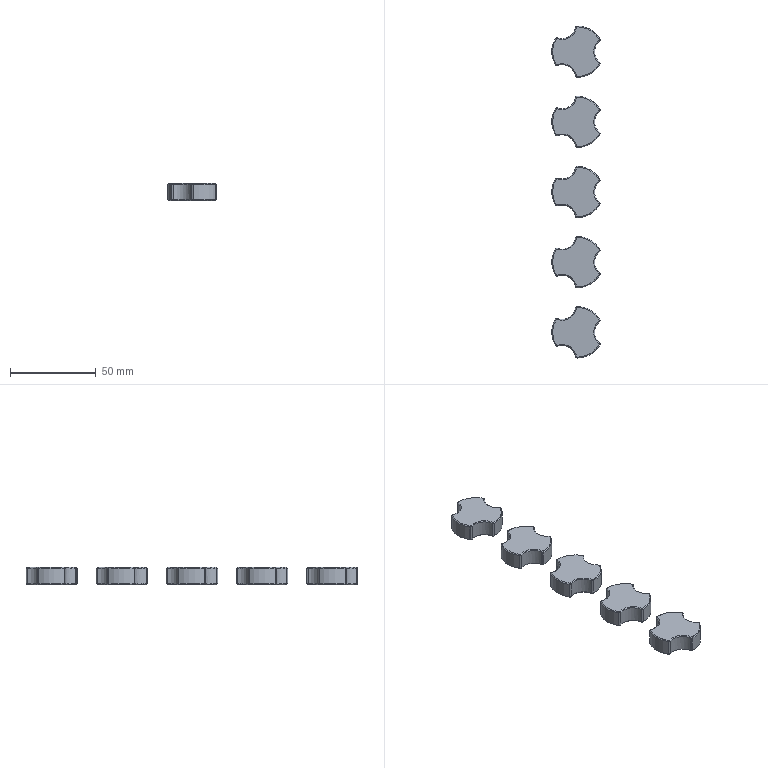NC program | NX | posted with a generic post | part box 28.194 x 194 x 10 mm
Lines 19 to 819 of 9608:
(ZLEVEL_PROFILE_COPY_1 , TOOL : D10)
N36 T15 M6
N38 G54
N40 G17 G0 G90 X-93.698 Y-15.206 S9500 M3
N42 G43 Z30. H15
N44 Z1.5
N46 G94 G1 X-93.806 Y-15.104 Z1.492 F1000.
N48 X-94.604 Y-13.894 Z1.416
N50 X-95.095 Y-12.53 Z1.34
N52 X-95.252 Y-11.089 Z1.264
N54 X-95.066 Y-9.651 Z1.188
N56 X-94.719 Y-8.688 Z1.135
N58 X-94.696 Y-7.629 Z1.079
N60 X-95.051 Y-6.632 Z1.024
N62 X-95.737 Y-5.826 Z0.968
N64 X-96.665 Y-5.317 Z0.913
N66 X-97.673 Y-5.136 Z0.859
N68 X-98.516 Y-4.828 Z0.812
N70 X-99.567 Y-4.224 Z0.749
N72 X-100.528 Y-3.37 Z0.681
N74 X-101.29 Y-2.334 Z0.614
N76 X-101.82 Y-1.162 Z0.546
N78 X-102.093 Y0.094 Z0.479
N80 X-102.099 Y0.7 Z0.447
N82 X-102.11 Y1.798 Z0.39
N84 X-101.8 Y4.534 Z0.245
N86 X-101.119 Y7.202 Z0.101
N88 X-100.081 Y9.752 Z-0.043
N90 X-98.704 Y12.136 Z-0.188
N92 X-97.015 Y14.311 Z-0.332
N94 X-95.045 Y16.234 Z-0.476
N96 X-92.831 Y17.871 Z-0.62
N98 X-91.346 Y18.708 Z-0.71
N100 X-89.833 Y19.152 Z-0.792
N102 X-88.256 Y19.196 Z-0.875
N104 X-86.721 Y18.836 Z-0.958
N106 X-86.179 Y18.565 Z-0.99
N108 X-86.089 Y18.522 Z-0.995
N110 X-86.001 Y18.476 Z-1.
N112 X-85.827 Y18.38 F3500.
N114 G2 X-84.216 Y17.032 R6.1
N116 G3 X-79.784 Y17.032 R2.9
N118 G2 X-72.126 Y18.411 R6.1
N120 X-61.901 Y0.7 R20.1
N122 X-66.924 Y-5.243 R6.1
N124 G3 X-69.14 Y-9.081 R2.9
N126 G2 X-71.775 Y-16.402 R6.1
N128 X-92.225 Y-16.402 R20.1
N130 X-94.86 Y-9.081 R6.1
N132 G3 X-97.076 Y-5.243 R2.9
N134 G2 X-102.099 Y0.7 R6.1
N136 X-91.874 Y18.411 R20.1
N138 X-86.179 Y18.565 R6.1
N140 G1 X-86.001 Y18.476
N142 X-85.914 Y18.429 Z-1.001
N144 X-85.827 Y18.38 Z-1.002
N146 X-85.382 Y18.097 Z-1.006
N148 X-84.963 Y17.776 Z-1.01
N150 X-84.573 Y17.42 Z-1.014
N152 X-84.216 Y17.032 Z-1.018
N154 X-84.043 Y16.845 Z-1.02
N156 X-83.855 Y16.674 Z-1.022
N158 X-83.597 Y16.482 Z-1.024
N160 X-83.437 Y16.384 Z-1.026
N162 X-82.986 Y16.175 Z-1.029
N164 X-82.691 Y16.086 Z-1.032
N166 X-82.222 Y16.011 Z-1.035
N168 X-81.893 Y16.005 Z-1.038
N170 X-81.425 Y16.06 Z-1.042
N172 X-81.103 Y16.145 Z-1.044
N174 X-80.669 Y16.326 Z-1.048
N176 X-80.382 Y16.496 Z-1.05
N178 X-80.064 Y16.743 Z-1.053
N180 X-79.784 Y17.032 Z-1.056
N182 X-79.373 Y17.473 Z-1.061
N184 X-78.921 Y17.871 Z-1.066
N186 X-78.431 Y18.222 Z-1.07
N188 X-77.91 Y18.523 Z-1.075
N190 X-77.361 Y18.772 Z-1.08
N192 X-76.79 Y18.965 Z-1.084
N194 X-76.203 Y19.101 Z-1.089
N196 X-75.606 Y19.178 Z-1.093
N198 X-75.004 Y19.196 Z-1.098
N200 X-74.403 Y19.155 Z-1.103
N202 X-73.809 Y19.054 Z-1.107
N204 X-73.228 Y18.895 Z-1.112
N206 X-72.665 Y18.68 Z-1.117
N208 X-72.126 Y18.411 Z-1.121
N210 X-71.206 Y17.859 Z-1.13
N212 X-70.317 Y17.259 Z-1.138
N214 X-69.461 Y16.612 Z-1.146
N216 X-68.641 Y15.921 Z-1.154
N218 X-67.859 Y15.187 Z-1.163
N220 X-67.117 Y14.413 Z-1.171
N222 X-66.418 Y13.599 Z-1.179
N224 X-65.763 Y12.75 Z-1.187
N226 X-65.154 Y11.867 Z-1.196
N228 X-64.593 Y10.953 Z-1.204
N230 X-64.082 Y10.01 Z-1.212
N232 X-63.621 Y9.041 Z-1.22
N234 X-63.213 Y8.049 Z-1.229
N236 X-62.859 Y7.037 Z-1.237
N238 X-62.559 Y6.007 Z-1.245
N240 X-62.314 Y4.963 Z-1.253
N242 X-62.126 Y3.907 Z-1.262
N244 X-61.994 Y2.842 Z-1.27
N246 X-61.919 Y1.772 Z-1.278
N248 X-61.901 Y0.7 Z-1.286
N250 X-61.937 Y0.098 Z-1.291
N252 X-62.032 Y-0.497 Z-1.296
N254 X-62.185 Y-1.079 Z-1.3
N256 X-62.395 Y-1.644 Z-1.305
N258 X-62.659 Y-2.185 Z-1.309
N260 X-62.976 Y-2.698 Z-1.314
N262 X-63.342 Y-3.176 Z-1.319
N264 X-63.753 Y-3.617 Z-1.323
N266 X-64.206 Y-4.014 Z-1.328
N268 X-64.695 Y-4.365 Z-1.333
N270 X-65.217 Y-4.666 Z-1.337
N272 X-65.766 Y-4.915 Z-1.342
N274 X-66.337 Y-5.107 Z-1.346
N276 X-66.924 Y-5.243 Z-1.351
N278 X-67.456 Y-5.392 Z-1.355
N280 X-67.61 Y-5.456 Z-1.357
N282 X-68. Y-5.671 Z-1.36
N284 X-68.223 Y-5.832 Z-1.362
N286 X-68.535 Y-6.123 Z-1.365
N288 X-68.724 Y-6.347 Z-1.368
N290 X-68.954 Y-6.702 Z-1.371
N292 X-69.083 Y-6.97 Z-1.373
N294 X-69.219 Y-7.369 Z-1.376
N296 X-69.279 Y-7.661 Z-1.379
N298 X-69.311 Y-8.082 Z-1.382
N300 X-69.298 Y-8.38 Z-1.384
N302 X-69.24 Y-8.735 Z-1.387
N304 X-69.14 Y-9.081 Z-1.39
N306 X-68.963 Y-9.657 Z-1.394
N308 X-68.845 Y-10.248 Z-1.399
N310 X-68.785 Y-10.847 Z-1.404
N312 Y-11.45 Z-1.408
N314 X-68.844 Y-12.049 Z-1.413
N316 X-68.963 Y-12.64 Z-1.418
N318 X-69.138 Y-13.216 Z-1.422
N320 X-69.37 Y-13.772 Z-1.427
N322 X-69.656 Y-14.303 Z-1.431
N324 X-69.992 Y-14.802 Z-1.436
N326 X-70.376 Y-15.267 Z-1.441
N328 X-70.804 Y-15.691 Z-1.445
N330 X-71.272 Y-16.07 Z-1.45
N332 X-71.775 Y-16.402 Z-1.455
N334 X-72.704 Y-16.918 Z-1.463
N336 X-73.66 Y-17.385 Z-1.471
N338 X-74.638 Y-17.801 Z-1.479
N340 X-75.638 Y-18.164 Z-1.487
N342 X-76.655 Y-18.474 Z-1.495
N344 X-77.687 Y-18.729 Z-1.504
N346 X-78.732 Y-18.93 Z-1.512
N348 X-79.785 Y-19.075 Z-1.52
N350 X-80.845 Y-19.164 Z-1.528
N352 X-81.907 Y-19.197 Z-1.536
N354 X-82.971 Y-19.174 Z-1.545
N356 X-84.031 Y-19.094 Z-1.553
N358 X-85.086 Y-18.959 Z-1.561
N360 X-86.132 Y-18.768 Z-1.569
N362 X-87.166 Y-18.522 Z-1.577
N364 X-88.186 Y-18.222 Z-1.585
N366 X-89.189 Y-17.868 Z-1.594
N368 X-90.172 Y-17.461 Z-1.602
N370 X-91.131 Y-17.003 Z-1.61
N372 X-92.065 Y-16.495 Z-1.618
N374 X-92.145 Y-16.449 Z-1.619
N376 X-92.225 Y-16.402 Z-1.62
N378 X-92.728 Y-16.07 Z-1.624
N380 X-93.196 Y-15.691 Z-1.629
N382 X-93.624 Y-15.267 Z-1.633
N384 X-94.008 Y-14.802 Z-1.638
N386 X-94.344 Y-14.303 Z-1.643
N388 X-94.63 Y-13.772 Z-1.647
N390 X-94.862 Y-13.216 Z-1.652
N392 X-95.037 Y-12.64 Z-1.657
N394 X-95.156 Y-12.049 Z-1.661
N396 X-95.215 Y-11.45 Z-1.666
N398 Y-10.847 Z-1.671
N400 X-95.155 Y-10.248 Z-1.675
N402 X-95.037 Y-9.657 Z-1.68
N404 X-94.86 Y-9.081 Z-1.684
N406 X-94.723 Y-8.545 Z-1.689
N408 X-94.702 Y-8.38 Z-1.69
N410 X-94.693 Y-7.935 Z-1.693
N412 X-94.721 Y-7.661 Z-1.695
N414 X-94.816 Y-7.245 Z-1.699
N416 X-94.917 Y-6.97 Z-1.701
N418 X-95.109 Y-6.593 Z-1.704
N420 X-95.276 Y-6.347 Z-1.707
N422 X-95.554 Y-6.03 Z-1.71
N424 X-95.777 Y-5.832 Z-1.712
N426 X-96.125 Y-5.594 Z-1.715
N428 X-96.39 Y-5.456 Z-1.718
N430 X-96.727 Y-5.328 Z-1.72
N432 X-97.076 Y-5.243 Z-1.723
N434 X-97.589 Y-5.128 Z-1.727
N436 X-98.09 Y-4.969 Z-1.731
N438 X-98.575 Y-4.768 Z-1.735
N440 X-99.041 Y-4.526 Z-1.739
N442 X-99.487 Y-4.243 Z-1.743
N444 X-99.907 Y-3.923 Z-1.747
N446 X-100.297 Y-3.568 Z-1.751
N448 X-100.655 Y-3.18 Z-1.755
N450 X-100.978 Y-2.763 Z-1.76
N452 X-101.264 Y-2.319 Z-1.764
N454 X-101.511 Y-1.853 Z-1.768
N456 X-101.716 Y-1.366 Z-1.772
N458 X-101.879 Y-0.864 Z-1.776
N460 X-101.997 Y-0.35 Z-1.78
N462 X-102.071 Y0.173 Z-1.784
N464 X-102.099 Y0.7 Z-1.788
N466 X-102.081 Y1.772 Z-1.796
N468 X-102.006 Y2.842 Z-1.804
N470 X-101.874 Y3.907 Z-1.813
N472 X-101.686 Y4.963 Z-1.821
N474 X-101.441 Y6.007 Z-1.829
N476 X-101.141 Y7.037 Z-1.837
N478 X-100.787 Y8.049 Z-1.846
N480 X-100.379 Y9.041 Z-1.854
N482 X-99.918 Y10.01 Z-1.862
N484 X-99.407 Y10.953 Z-1.87
N486 X-98.846 Y11.867 Z-1.879
N488 X-98.237 Y12.75 Z-1.887
N490 X-97.582 Y13.599 Z-1.895
N492 X-96.883 Y14.413 Z-1.903
N494 X-96.141 Y15.187 Z-1.912
N496 X-95.359 Y15.921 Z-1.92
N498 X-94.539 Y16.612 Z-1.928
N500 X-93.683 Y17.259 Z-1.936
N502 X-92.794 Y17.859 Z-1.945
N504 X-91.874 Y18.411 Z-1.953
N506 X-91.344 Y18.676 Z-1.957
N508 X-90.791 Y18.889 Z-1.962
N510 X-90.22 Y19.048 Z-1.967
N512 X-89.636 Y19.15 Z-1.971
N514 X-89.045 Y19.195 Z-1.976
N516 X-88.453 Y19.182 Z-1.98
N518 X-87.864 Y19.113 Z-1.985
N520 X-87.285 Y18.986 Z-1.989
N522 X-86.709 Y18.799 Z-1.994
N524 X-86.176 Y18.566 Z-1.998
N526 X-86.088 Y18.522 Z-1.999
N528 X-86.001 Y18.476 Z-2.
N530 X-85.914 Y18.429 Z-2.001
N532 X-85.827 Y18.38 Z-2.002
N534 X-85.382 Y18.097 Z-2.006
N536 X-84.963 Y17.776 Z-2.01
N538 X-84.573 Y17.42 Z-2.014
N540 X-84.216 Y17.032 Z-2.018
N542 X-84.043 Y16.845 Z-2.02
N544 X-83.855 Y16.674 Z-2.022
N546 X-83.597 Y16.482 Z-2.024
N548 X-83.437 Y16.384 Z-2.026
N550 X-82.986 Y16.175 Z-2.029
N552 X-82.691 Y16.086 Z-2.032
N554 X-82.222 Y16.011 Z-2.035
N556 X-81.893 Y16.005 Z-2.038
N558 X-81.425 Y16.06 Z-2.042
N560 X-81.103 Y16.145 Z-2.044
N562 X-80.669 Y16.326 Z-2.048
N564 X-80.382 Y16.496 Z-2.05
N566 X-80.064 Y16.743 Z-2.053
N568 X-79.784 Y17.032 Z-2.056
N570 X-79.373 Y17.473 Z-2.061
N572 X-78.921 Y17.871 Z-2.066
N574 X-78.431 Y18.222 Z-2.07
N576 X-77.91 Y18.523 Z-2.075
N578 X-77.361 Y18.772 Z-2.08
N580 X-76.79 Y18.965 Z-2.084
N582 X-76.203 Y19.101 Z-2.089
N584 X-75.606 Y19.178 Z-2.093
N586 X-75.004 Y19.196 Z-2.098
N588 X-74.403 Y19.155 Z-2.103
N590 X-73.809 Y19.054 Z-2.107
N592 X-73.228 Y18.895 Z-2.112
N594 X-72.665 Y18.68 Z-2.117
N596 X-72.126 Y18.411 Z-2.121
N598 X-71.206 Y17.859 Z-2.13
N600 X-70.317 Y17.259 Z-2.138
N602 X-69.461 Y16.612 Z-2.146
N604 X-68.641 Y15.921 Z-2.154
N606 X-67.859 Y15.187 Z-2.163
N608 X-67.117 Y14.413 Z-2.171
N610 X-66.418 Y13.599 Z-2.179
N612 X-65.763 Y12.75 Z-2.187
N614 X-65.154 Y11.867 Z-2.196
N616 X-64.593 Y10.953 Z-2.204
N618 X-64.082 Y10.01 Z-2.212
N620 X-63.621 Y9.041 Z-2.22
N622 X-63.213 Y8.049 Z-2.229
N624 X-62.859 Y7.037 Z-2.237
N626 X-62.559 Y6.007 Z-2.245
N628 X-62.314 Y4.963 Z-2.253
N630 X-62.126 Y3.907 Z-2.262
N632 X-61.994 Y2.842 Z-2.27
N634 X-61.919 Y1.772 Z-2.278
N636 X-61.901 Y0.7 Z-2.286
N638 X-61.937 Y0.098 Z-2.291
N640 X-62.032 Y-0.497 Z-2.296
N642 X-62.185 Y-1.079 Z-2.3
N644 X-62.395 Y-1.644 Z-2.305
N646 X-62.659 Y-2.185 Z-2.309
N648 X-62.976 Y-2.698 Z-2.314
N650 X-63.342 Y-3.176 Z-2.319
N652 X-63.753 Y-3.617 Z-2.323
N654 X-64.206 Y-4.014 Z-2.328
N656 X-64.695 Y-4.365 Z-2.333
N658 X-65.217 Y-4.666 Z-2.337
N660 X-65.766 Y-4.915 Z-2.342
N662 X-66.337 Y-5.107 Z-2.346
N664 X-66.924 Y-5.243 Z-2.351
N666 X-67.456 Y-5.392 Z-2.355
N668 X-67.61 Y-5.456 Z-2.357
N670 X-68. Y-5.671 Z-2.36
N672 X-68.223 Y-5.832 Z-2.362
N674 X-68.535 Y-6.123 Z-2.365
N676 X-68.724 Y-6.347 Z-2.368
N678 X-68.954 Y-6.702 Z-2.371
N680 X-69.083 Y-6.97 Z-2.373
N682 X-69.219 Y-7.369 Z-2.376
N684 X-69.279 Y-7.661 Z-2.379
N686 X-69.311 Y-8.082 Z-2.382
N688 X-69.298 Y-8.38 Z-2.384
N690 X-69.24 Y-8.735 Z-2.387
N692 X-69.14 Y-9.081 Z-2.39
N694 X-68.963 Y-9.657 Z-2.394
N696 X-68.845 Y-10.248 Z-2.399
N698 X-68.785 Y-10.847 Z-2.404
N700 Y-11.45 Z-2.408
N702 X-68.844 Y-12.049 Z-2.413
N704 X-68.963 Y-12.64 Z-2.418
N706 X-69.138 Y-13.216 Z-2.422
N708 X-69.37 Y-13.772 Z-2.427
N710 X-69.656 Y-14.303 Z-2.431
N712 X-69.992 Y-14.802 Z-2.436
N714 X-70.376 Y-15.267 Z-2.441
N716 X-70.804 Y-15.691 Z-2.445
N718 X-71.272 Y-16.07 Z-2.45
N720 X-71.775 Y-16.402 Z-2.455
N722 X-72.704 Y-16.918 Z-2.463
N724 X-73.66 Y-17.385 Z-2.471
N726 X-74.638 Y-17.801 Z-2.479
N728 X-75.638 Y-18.164 Z-2.487
N730 X-76.655 Y-18.474 Z-2.495
N732 X-77.687 Y-18.729 Z-2.504
N734 X-78.732 Y-18.93 Z-2.512
N736 X-79.785 Y-19.075 Z-2.52
N738 X-80.845 Y-19.164 Z-2.528
N740 X-81.907 Y-19.197 Z-2.536
N742 X-82.971 Y-19.174 Z-2.545
N744 X-84.031 Y-19.094 Z-2.553
N746 X-85.086 Y-18.959 Z-2.561
N748 X-86.132 Y-18.768 Z-2.569
N750 X-87.166 Y-18.522 Z-2.577
N752 X-88.186 Y-18.222 Z-2.585
N754 X-89.189 Y-17.868 Z-2.594
N756 X-90.172 Y-17.461 Z-2.602
N758 X-91.131 Y-17.003 Z-2.61
N760 X-92.065 Y-16.495 Z-2.618
N762 X-92.145 Y-16.449 Z-2.619
N764 X-92.225 Y-16.402 Z-2.62
N766 X-92.728 Y-16.07 Z-2.624
N768 X-93.196 Y-15.691 Z-2.629
N770 X-93.624 Y-15.267 Z-2.633
N772 X-94.008 Y-14.802 Z-2.638
N774 X-94.344 Y-14.303 Z-2.643
N776 X-94.63 Y-13.772 Z-2.647
N778 X-94.862 Y-13.216 Z-2.652
N780 X-95.037 Y-12.64 Z-2.657
N782 X-95.156 Y-12.049 Z-2.661
N784 X-95.215 Y-11.45 Z-2.666
N786 Y-10.847 Z-2.671
N788 X-95.155 Y-10.248 Z-2.675
N790 X-95.037 Y-9.657 Z-2.68
N792 X-94.86 Y-9.081 Z-2.684
N794 X-94.723 Y-8.545 Z-2.689
N796 X-94.702 Y-8.38 Z-2.69
N798 X-94.693 Y-7.935 Z-2.693
N800 X-94.721 Y-7.661 Z-2.695
N802 X-94.816 Y-7.245 Z-2.699
N804 X-94.917 Y-6.97 Z-2.701
N806 X-95.109 Y-6.593 Z-2.704
N808 X-95.276 Y-6.347 Z-2.707
N810 X-95.554 Y-6.03 Z-2.71
N812 X-95.777 Y-5.832 Z-2.712
N814 X-96.125 Y-5.594 Z-2.715
N816 X-96.39 Y-5.456 Z-2.718
N818 X-96.727 Y-5.328 Z-2.72
N820 X-97.076 Y-5.243 Z-2.723
N822 X-97.589 Y-5.128 Z-2.727
N824 X-98.09 Y-4.969 Z-2.731
N826 X-98.575 Y-4.768 Z-2.735
N828 X-99.041 Y-4.526 Z-2.739
N830 X-99.487 Y-4.243 Z-2.743
N832 X-99.907 Y-3.923 Z-2.747
N834 X-100.297 Y-3.568 Z-2.751
N836 X-100.655 Y-3.18 Z-2.755
N838 X-100.978 Y-2.763 Z-2.76
N840 X-101.264 Y-2.319 Z-2.764
N842 X-101.511 Y-1.853 Z-2.768
N844 X-101.716 Y-1.366 Z-2.772
N846 X-101.879 Y-0.864 Z-2.776
N848 X-101.997 Y-0.35 Z-2.78
N850 X-102.071 Y0.173 Z-2.784
N852 X-102.099 Y0.7 Z-2.788
N854 X-102.081 Y1.772 Z-2.796
N856 X-102.006 Y2.842 Z-2.804
N858 X-101.874 Y3.907 Z-2.813
N860 X-101.686 Y4.963 Z-2.821
N862 X-101.441 Y6.007 Z-2.829
N864 X-101.141 Y7.037 Z-2.837
N866 X-100.787 Y8.049 Z-2.846
N868 X-100.379 Y9.041 Z-2.854
N870 X-99.918 Y10.01 Z-2.862
N872 X-99.407 Y10.953 Z-2.87
N874 X-98.846 Y11.867 Z-2.879
N876 X-98.237 Y12.75 Z-2.887
N878 X-97.582 Y13.599 Z-2.895
N880 X-96.883 Y14.413 Z-2.903
N882 X-96.141 Y15.187 Z-2.912
N884 X-95.359 Y15.921 Z-2.92
N886 X-94.539 Y16.612 Z-2.928
N888 X-93.683 Y17.259 Z-2.936
N890 X-92.794 Y17.859 Z-2.945
N892 X-91.874 Y18.411 Z-2.953
N894 X-91.344 Y18.676 Z-2.957
N896 X-90.791 Y18.889 Z-2.962
N898 X-90.22 Y19.048 Z-2.967
N900 X-89.636 Y19.15 Z-2.971
N902 X-89.045 Y19.195 Z-2.976
N904 X-88.453 Y19.182 Z-2.98
N906 X-87.864 Y19.113 Z-2.985
N908 X-87.285 Y18.986 Z-2.989
N910 X-86.709 Y18.799 Z-2.994
N912 X-86.176 Y18.566 Z-2.998
N914 X-86.088 Y18.522 Z-2.999
N916 X-86.001 Y18.476 Z-3.
N918 X-85.914 Y18.429 Z-3.001
N920 X-85.827 Y18.38 Z-3.002
N922 X-85.382 Y18.097 Z-3.006
N924 X-84.963 Y17.776 Z-3.01
N926 X-84.573 Y17.42 Z-3.014
N928 X-84.216 Y17.032 Z-3.018
N930 X-84.043 Y16.845 Z-3.02
N932 X-83.855 Y16.674 Z-3.022
N934 X-83.597 Y16.482 Z-3.024
N936 X-83.437 Y16.384 Z-3.026
N938 X-82.986 Y16.175 Z-3.029
N940 X-82.691 Y16.086 Z-3.032
N942 X-82.222 Y16.011 Z-3.035
N944 X-81.893 Y16.005 Z-3.038
N946 X-81.425 Y16.06 Z-3.042
N948 X-81.103 Y16.145 Z-3.044
N950 X-80.669 Y16.326 Z-3.048
N952 X-80.382 Y16.496 Z-3.05
N954 X-80.064 Y16.743 Z-3.053
N956 X-79.784 Y17.032 Z-3.056
N958 X-79.373 Y17.473 Z-3.061
N960 X-78.921 Y17.871 Z-3.066
N962 X-78.431 Y18.222 Z-3.07
N964 X-77.91 Y18.523 Z-3.075
N966 X-77.361 Y18.772 Z-3.08
N968 X-76.79 Y18.965 Z-3.084
N970 X-76.203 Y19.101 Z-3.089
N972 X-75.606 Y19.178 Z-3.093
N974 X-75.004 Y19.196 Z-3.098
N976 X-74.403 Y19.155 Z-3.103
N978 X-73.809 Y19.054 Z-3.107
N980 X-73.228 Y18.895 Z-3.112
N982 X-72.665 Y18.68 Z-3.117
N984 X-72.126 Y18.411 Z-3.121
N986 X-71.206 Y17.859 Z-3.13
N988 X-70.317 Y17.259 Z-3.138
N990 X-69.461 Y16.612 Z-3.146
N992 X-68.641 Y15.921 Z-3.154
N994 X-67.859 Y15.187 Z-3.163
N996 X-67.117 Y14.413 Z-3.171
N998 X-66.418 Y13.599 Z-3.179
N1000 X-65.763 Y12.75 Z-3.187
N1002 X-65.154 Y11.867 Z-3.196
N1004 X-64.593 Y10.953 Z-3.204
N1006 X-64.082 Y10.01 Z-3.212
N1008 X-63.621 Y9.041 Z-3.22
N1010 X-63.213 Y8.049 Z-3.229
N1012 X-62.859 Y7.037 Z-3.237
N1014 X-62.559 Y6.007 Z-3.245
N1016 X-62.314 Y4.963 Z-3.253
N1018 X-62.126 Y3.907 Z-3.262
N1020 X-61.994 Y2.842 Z-3.27
N1022 X-61.919 Y1.772 Z-3.278
N1024 X-61.901 Y0.7 Z-3.286
N1026 X-61.937 Y0.098 Z-3.291
N1028 X-62.032 Y-0.497 Z-3.296
N1030 X-62.185 Y-1.079 Z-3.3
N1032 X-62.395 Y-1.644 Z-3.305
N1034 X-62.659 Y-2.185 Z-3.309
N1036 X-62.976 Y-2.698 Z-3.314
N1038 X-63.342 Y-3.176 Z-3.319
N1040 X-63.753 Y-3.617 Z-3.323
N1042 X-64.206 Y-4.014 Z-3.328
N1044 X-64.695 Y-4.365 Z-3.333
N1046 X-65.217 Y-4.666 Z-3.337
N1048 X-65.766 Y-4.915 Z-3.342
N1050 X-66.337 Y-5.107 Z-3.346
N1052 X-66.924 Y-5.243 Z-3.351
N1054 X-67.456 Y-5.392 Z-3.355
N1056 X-67.61 Y-5.456 Z-3.357
N1058 X-68. Y-5.671 Z-3.36
N1060 X-68.223 Y-5.832 Z-3.362
N1062 X-68.535 Y-6.123 Z-3.365
N1064 X-68.724 Y-6.347 Z-3.368
N1066 X-68.954 Y-6.702 Z-3.371
N1068 X-69.083 Y-6.97 Z-3.373
N1070 X-69.219 Y-7.369 Z-3.376
N1072 X-69.279 Y-7.661 Z-3.379
N1074 X-69.311 Y-8.082 Z-3.382
N1076 X-69.298 Y-8.38 Z-3.384
N1078 X-69.24 Y-8.735 Z-3.387
N1080 X-69.14 Y-9.081 Z-3.39
N1082 X-68.963 Y-9.657 Z-3.394
N1084 X-68.845 Y-10.248 Z-3.399
N1086 X-68.785 Y-10.847 Z-3.404
N1088 Y-11.45 Z-3.408
N1090 X-68.844 Y-12.049 Z-3.413
N1092 X-68.963 Y-12.64 Z-3.418
N1094 X-69.138 Y-13.216 Z-3.422
N1096 X-69.37 Y-13.772 Z-3.427
N1098 X-69.656 Y-14.303 Z-3.431
N1100 X-69.992 Y-14.802 Z-3.436
N1102 X-70.376 Y-15.267 Z-3.441
N1104 X-70.804 Y-15.691 Z-3.445
N1106 X-71.272 Y-16.07 Z-3.45
N1108 X-71.775 Y-16.402 Z-3.455
N1110 X-72.704 Y-16.918 Z-3.463
N1112 X-73.66 Y-17.385 Z-3.471
N1114 X-74.638 Y-17.801 Z-3.479
N1116 X-75.638 Y-18.164 Z-3.487
N1118 X-76.655 Y-18.474 Z-3.495
N1120 X-77.687 Y-18.729 Z-3.504
N1122 X-78.732 Y-18.93 Z-3.512
N1124 X-79.785 Y-19.075 Z-3.52
N1126 X-80.845 Y-19.164 Z-3.528
N1128 X-81.907 Y-19.197 Z-3.536
N1130 X-82.971 Y-19.174 Z-3.545
N1132 X-84.031 Y-19.094 Z-3.553
N1134 X-85.086 Y-18.959 Z-3.561
N1136 X-86.132 Y-18.768 Z-3.569
N1138 X-87.166 Y-18.522 Z-3.577
N1140 X-88.186 Y-18.222 Z-3.585
N1142 X-89.189 Y-17.868 Z-3.594
N1144 X-90.172 Y-17.461 Z-3.602
N1146 X-91.131 Y-17.003 Z-3.61
N1148 X-92.065 Y-16.495 Z-3.618
N1150 X-92.145 Y-16.449 Z-3.619
N1152 X-92.225 Y-16.402 Z-3.62
N1154 X-92.728 Y-16.07 Z-3.624
N1156 X-93.196 Y-15.691 Z-3.629
N1158 X-93.624 Y-15.267 Z-3.633
N1160 X-94.008 Y-14.802 Z-3.638
N1162 X-94.344 Y-14.303 Z-3.643
N1164 X-94.63 Y-13.772 Z-3.647
N1166 X-94.862 Y-13.216 Z-3.652
N1168 X-95.037 Y-12.64 Z-3.657
N1170 X-95.156 Y-12.049 Z-3.661
N1172 X-95.215 Y-11.45 Z-3.666
N1174 Y-10.847 Z-3.671
N1176 X-95.155 Y-10.248 Z-3.675
N1178 X-95.037 Y-9.657 Z-3.68
N1180 X-94.86 Y-9.081 Z-3.684
N1182 X-94.723 Y-8.545 Z-3.689
N1184 X-94.702 Y-8.38 Z-3.69
N1186 X-94.693 Y-7.935 Z-3.693
N1188 X-94.721 Y-7.661 Z-3.695
N1190 X-94.816 Y-7.245 Z-3.699
N1192 X-94.917 Y-6.97 Z-3.701
N1194 X-95.109 Y-6.593 Z-3.704
N1196 X-95.276 Y-6.347 Z-3.707
N1198 X-95.554 Y-6.03 Z-3.71
N1200 X-95.777 Y-5.832 Z-3.712
N1202 X-96.125 Y-5.594 Z-3.715
N1204 X-96.39 Y-5.456 Z-3.718
N1206 X-96.727 Y-5.328 Z-3.72
N1208 X-97.076 Y-5.243 Z-3.723
N1210 X-97.589 Y-5.128 Z-3.727
N1212 X-98.09 Y-4.969 Z-3.731
N1214 X-98.575 Y-4.768 Z-3.735
N1216 X-99.041 Y-4.526 Z-3.739
N1218 X-99.487 Y-4.243 Z-3.743
N1220 X-99.907 Y-3.923 Z-3.747
N1222 X-100.297 Y-3.568 Z-3.751
N1224 X-100.655 Y-3.18 Z-3.755
N1226 X-100.978 Y-2.763 Z-3.76
N1228 X-101.264 Y-2.319 Z-3.764
N1230 X-101.511 Y-1.853 Z-3.768
N1232 X-101.716 Y-1.366 Z-3.772
N1234 X-101.879 Y-0.864 Z-3.776
N1236 X-101.997 Y-0.35 Z-3.78
N1238 X-102.071 Y0.173 Z-3.784
N1240 X-102.099 Y0.7 Z-3.788
N1242 X-102.081 Y1.772 Z-3.796
N1244 X-102.006 Y2.842 Z-3.804
N1246 X-101.874 Y3.907 Z-3.813
N1248 X-101.686 Y4.963 Z-3.821
N1250 X-101.441 Y6.007 Z-3.829
N1252 X-101.141 Y7.037 Z-3.837
N1254 X-100.787 Y8.049 Z-3.846
N1256 X-100.379 Y9.041 Z-3.854
N1258 X-99.918 Y10.01 Z-3.862
N1260 X-99.407 Y10.953 Z-3.87
N1262 X-98.846 Y11.867 Z-3.879
N1264 X-98.237 Y12.75 Z-3.887
N1266 X-97.582 Y13.599 Z-3.895
N1268 X-96.883 Y14.413 Z-3.903
N1270 X-96.141 Y15.187 Z-3.912
N1272 X-95.359 Y15.921 Z-3.92
N1274 X-94.539 Y16.612 Z-3.928
N1276 X-93.683 Y17.259 Z-3.936
N1278 X-92.794 Y17.859 Z-3.945
N1280 X-91.874 Y18.411 Z-3.953
N1282 X-91.344 Y18.676 Z-3.957
N1284 X-90.791 Y18.889 Z-3.962
N1286 X-90.22 Y19.048 Z-3.967
N1288 X-89.636 Y19.15 Z-3.971
N1290 X-89.045 Y19.195 Z-3.976
N1292 X-88.453 Y19.182 Z-3.98
N1294 X-87.864 Y19.113 Z-3.985
N1296 X-87.285 Y18.986 Z-3.989
N1298 X-86.709 Y18.799 Z-3.994
N1300 X-86.176 Y18.566 Z-3.998
N1302 X-86.088 Y18.522 Z-3.999
N1304 X-86.001 Y18.476 Z-4.
N1306 X-85.914 Y18.429 Z-4.001
N1308 X-85.827 Y18.38 Z-4.002
N1310 X-85.382 Y18.097 Z-4.006
N1312 X-84.963 Y17.776 Z-4.01
N1314 X-84.573 Y17.42 Z-4.014
N1316 X-84.216 Y17.032 Z-4.018
N1318 X-84.043 Y16.845 Z-4.02
N1320 X-83.855 Y16.674 Z-4.022
N1322 X-83.597 Y16.482 Z-4.024
N1324 X-83.437 Y16.384 Z-4.026
N1326 X-82.986 Y16.175 Z-4.029
N1328 X-82.691 Y16.086 Z-4.032
N1330 X-82.222 Y16.011 Z-4.035
N1332 X-81.893 Y16.005 Z-4.038
N1334 X-81.425 Y16.06 Z-4.042
N1336 X-81.103 Y16.145 Z-4.044
N1338 X-80.669 Y16.326 Z-4.048
N1340 X-80.382 Y16.496 Z-4.05
N1342 X-80.064 Y16.743 Z-4.053
N1344 X-79.784 Y17.032 Z-4.056
N1346 X-79.373 Y17.473 Z-4.061
N1348 X-78.921 Y17.871 Z-4.066
N1350 X-78.431 Y18.222 Z-4.07
N1352 X-77.91 Y18.523 Z-4.075
N1354 X-77.361 Y18.772 Z-4.08
N1356 X-76.79 Y18.965 Z-4.084
N1358 X-76.203 Y19.101 Z-4.089
N1360 X-75.606 Y19.178 Z-4.093
N1362 X-75.004 Y19.196 Z-4.098
N1364 X-74.403 Y19.155 Z-4.103
N1366 X-73.809 Y19.054 Z-4.107
N1368 X-73.228 Y18.895 Z-4.112
N1370 X-72.665 Y18.68 Z-4.117
N1372 X-72.126 Y18.411 Z-4.121
N1374 X-71.206 Y17.859 Z-4.13
N1376 X-70.317 Y17.259 Z-4.138
N1378 X-69.461 Y16.612 Z-4.146
N1380 X-68.641 Y15.921 Z-4.154
N1382 X-67.859 Y15.187 Z-4.163
N1384 X-67.117 Y14.413 Z-4.171
N1386 X-66.418 Y13.599 Z-4.179
N1388 X-65.763 Y12.75 Z-4.187
N1390 X-65.154 Y11.867 Z-4.196
N1392 X-64.593 Y10.953 Z-4.204
N1394 X-64.082 Y10.01 Z-4.212
N1396 X-63.621 Y9.041 Z-4.22
N1398 X-63.213 Y8.049 Z-4.229
N1400 X-62.859 Y7.037 Z-4.237
N1402 X-62.559 Y6.007 Z-4.245
N1404 X-62.314 Y4.963 Z-4.253
N1406 X-62.126 Y3.907 Z-4.262
N1408 X-61.994 Y2.842 Z-4.27
N1410 X-61.919 Y1.772 Z-4.278
N1412 X-61.901 Y0.7 Z-4.286
N1414 X-61.937 Y0.098 Z-4.291
N1416 X-62.032 Y-0.497 Z-4.296
N1418 X-62.185 Y-1.079 Z-4.3
N1420 X-62.395 Y-1.644 Z-4.305
N1422 X-62.659 Y-2.185 Z-4.309
N1424 X-62.976 Y-2.698 Z-4.314
N1426 X-63.342 Y-3.176 Z-4.319
N1428 X-63.753 Y-3.617 Z-4.323
N1430 X-64.206 Y-4.014 Z-4.328
N1432 X-64.695 Y-4.365 Z-4.333
N1434 X-65.217 Y-4.666 Z-4.337
N1436 X-65.766 Y-4.915 Z-4.342
N1438 X-66.337 Y-5.107 Z-4.346
N1440 X-66.924 Y-5.243 Z-4.351
N1442 X-67.456 Y-5.392 Z-4.355
N1444 X-67.61 Y-5.456 Z-4.357
N1446 X-68. Y-5.671 Z-4.36
N1448 X-68.223 Y-5.832 Z-4.362
N1450 X-68.535 Y-6.123 Z-4.365
N1452 X-68.724 Y-6.347 Z-4.368
N1454 X-68.954 Y-6.702 Z-4.371
N1456 X-69.083 Y-6.97 Z-4.373
N1458 X-69.219 Y-7.369 Z-4.376
N1460 X-69.279 Y-7.661 Z-4.379
N1462 X-69.311 Y-8.082 Z-4.382
N1464 X-69.298 Y-8.38 Z-4.384
N1466 X-69.24 Y-8.735 Z-4.387
N1468 X-69.14 Y-9.081 Z-4.39
N1470 X-68.963 Y-9.657 Z-4.394
N1472 X-68.845 Y-10.248 Z-4.399
N1474 X-68.785 Y-10.847 Z-4.404
N1476 Y-11.45 Z-4.408
N1478 X-68.844 Y-12.049 Z-4.413
N1480 X-68.963 Y-12.64 Z-4.418
N1482 X-69.138 Y-13.216 Z-4.422
N1484 X-69.37 Y-13.772 Z-4.427
N1486 X-69.656 Y-14.303 Z-4.431
N1488 X-69.992 Y-14.802 Z-4.436
N1490 X-70.376 Y-15.267 Z-4.441
N1492 X-70.804 Y-15.691 Z-4.445
N1494 X-71.272 Y-16.07 Z-4.45
N1496 X-71.775 Y-16.402 Z-4.455
N1498 X-72.704 Y-16.918 Z-4.463
N1500 X-73.66 Y-17.385 Z-4.471
N1502 X-74.638 Y-17.801 Z-4.479
N1504 X-75.638 Y-18.164 Z-4.487
N1506 X-76.655 Y-18.474 Z-4.495
N1508 X-77.687 Y-18.729 Z-4.504
N1510 X-78.732 Y-18.93 Z-4.512
N1512 X-79.785 Y-19.075 Z-4.52
N1514 X-80.845 Y-19.164 Z-4.528
N1516 X-81.907 Y-19.197 Z-4.536
N1518 X-82.971 Y-19.174 Z-4.545
N1520 X-84.031 Y-19.094 Z-4.553
N1522 X-85.086 Y-18.959 Z-4.561
N1524 X-86.132 Y-18.768 Z-4.569
N1526 X-87.166 Y-18.522 Z-4.577
N1528 X-88.186 Y-18.222 Z-4.585
N1530 X-89.189 Y-17.868 Z-4.594
N1532 X-90.172 Y-17.461 Z-4.602
N1534 X-91.131 Y-17.003 Z-4.61
N1536 X-92.065 Y-16.495 Z-4.618
N1538 X-92.145 Y-16.449 Z-4.619
N1540 X-92.225 Y-16.402 Z-4.62
N1542 X-92.728 Y-16.07 Z-4.624
N1544 X-93.196 Y-15.691 Z-4.629
N1546 X-93.624 Y-15.267 Z-4.633
N1548 X-94.008 Y-14.802 Z-4.638
N1550 X-94.344 Y-14.303 Z-4.643
N1552 X-94.63 Y-13.772 Z-4.647
N1554 X-94.862 Y-13.216 Z-4.652
N1556 X-95.037 Y-12.64 Z-4.657
N1558 X-95.156 Y-12.049 Z-4.661
N1560 X-95.215 Y-11.45 Z-4.666
N1562 Y-10.847 Z-4.671
N1564 X-95.155 Y-10.248 Z-4.675
N1566 X-95.037 Y-9.657 Z-4.68
N1568 X-94.86 Y-9.081 Z-4.684
N1570 X-94.723 Y-8.545 Z-4.689
N1572 X-94.702 Y-8.38 Z-4.69
N1574 X-94.693 Y-7.935 Z-4.693
N1576 X-94.721 Y-7.661 Z-4.695
N1578 X-94.816 Y-7.245 Z-4.699
N1580 X-94.917 Y-6.97 Z-4.701
N1582 X-95.109 Y-6.593 Z-4.704
N1584 X-95.276 Y-6.347 Z-4.707
N1586 X-95.554 Y-6.03 Z-4.71
N1588 X-95.777 Y-5.832 Z-4.712
N1590 X-96.125 Y-5.594 Z-4.715
N1592 X-96.39 Y-5.456 Z-4.718
N1594 X-96.727 Y-5.328 Z-4.72
N1596 X-97.076 Y-5.243 Z-4.723
N1598 X-97.589 Y-5.128 Z-4.727
N1600 X-98.09 Y-4.969 Z-4.731
N1602 X-98.575 Y-4.768 Z-4.735
N1604 X-99.041 Y-4.526 Z-4.739
N1606 X-99.487 Y-4.243 Z-4.743
N1608 X-99.907 Y-3.923 Z-4.747
N1610 X-100.297 Y-3.568 Z-4.751
N1612 X-100.655 Y-3.18 Z-4.755
N1614 X-100.978 Y-2.763 Z-4.76
N1616 X-101.264 Y-2.319 Z-4.764
N1618 X-101.511 Y-1.853 Z-4.768
N1620 X-101.716 Y-1.366 Z-4.772
N1622 X-101.879 Y-0.864 Z-4.776
N1624 X-101.997 Y-0.35 Z-4.78
N1626 X-102.071 Y0.173 Z-4.784
N1628 X-102.099 Y0.7 Z-4.788
N1630 X-102.081 Y1.772 Z-4.796